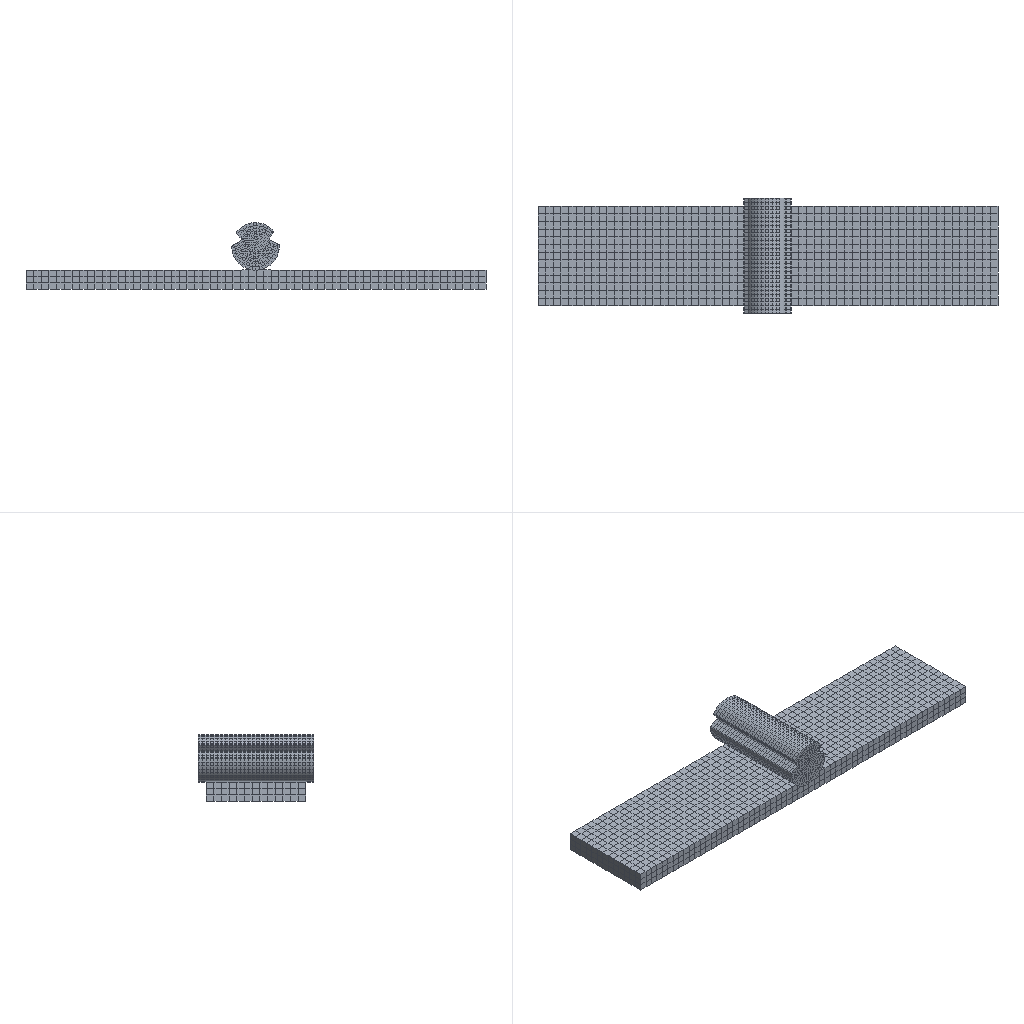Simulation study | abaqus
Set-up summary:
category,name,step,type,value,unit,region
solver,abaqus
solver,version,,,Abaqus/Standard 2020
units,not stated in the deck,,not stated
analysis,deck,,static,static
load_step,Step-1,Step-1,static
load_step,requested,,,1
mesh,nodes,,,13088
mesh,elements,,,10920
element_type,C3D8R,,solid,10920
load,load commands in deck,,count,1
bc,support commands in deck,,count,6
material,TAN,,in results
material,XIAN,,in results
check,setup vs results,,match,"per instance, exact: element labels, types and connectivity; labels of the nodes the elements use; coordinates not compared"
Abaqus input file, long lists of numbers shortened:
*Heading
** Job name: Job-2 Model name: Model-2
** Generated by: Abaqus/CAE 2020
*Preprint, echo=NO, model=NO, history=NO, contact=NO
**
** PARTS
**
*Part, name=P222
*Node
      1,         120.,         -23.,           5.
      2,         120.,         -23.,   3.333
** (3414 more lines like these left out)
*Element, type=C3D8R
   1,   57,   58,   62,   61,    1,    2,    6,    5
   2,   58,   59,   63,   62,    2,    3,    7,    6
** (2338 more lines like these left out)
*Nset, nset=Set-2, generate
    1,  3416,     1
*Elset, elset=Set-2, generate
    1,  2340,     1
** Section: tan
*Solid Section, elset=Set-2, material=tan
,
*End Part
**
*Part, name=dao
*Node
      1,   -6.104,  0.109,           0.
      2,  -5.946,  0.3737,           0.
** (9670 more lines like these left out)
*Element, type=C3D8R
   1,  164,  141,  127,  162,  476,  453,  439,  474
   2,  276,  162,  127,  277,  588,  474,  439,  589
** (8578 more lines like these left out)
*Nset, nset=Set-2, generate
    1,  9672,     1
*Elset, elset=Set-2, generate
    1,  8580,     1
** Section: xian
*Solid Section, elset=Set-2, material=xian
,
*End Part
**
**
** ASSEMBLY
**
*Assembly, name=Assembly
**
*Instance, name=P222-1, part=P222
*End Instance
**
*Instance, name=dao-1, part=dao
   59.767,           5.,    11.079
   59.767,           5.,    11.079, 60.767,           5.,    11.079, 90.
*End Instance
**
*Nset, nset=Set-1, instance=P222-1, generate
    1,  3416,     1
*Nset, nset=Set-1, instance=dao-1, generate
    1,  9672,     1
*Elset, elset=Set-1, instance=P222-1, generate
    1,  2340,     1
*Elset, elset=Set-1, instance=dao-1, generate
    1,  8580,     1
*Nset, nset=Set-2, instance=dao-1
    2,    3,    5,    6,   16,   17,   19,   20,   33,   34,   40,   41,  314,  315,  317,  318
  328,  329,  331,  332,  345,  346,  352,  353,  626,  627,  629,  630,  640,  641,  643,  644
** (22 more lines like these left out)
*Elset, elset=Set-2, instance=dao-1
   11,   28,   40,   89,   94,  175,  203,  273,  297,  314,  326,  375,  380,  461,  489,  559
  583,  600,  612,  661,  666,  747,  775,  845,  869,  886,  898,  947,  952, 1033, 1061, 1131
** (13 more lines like these left out)
*Nset, nset=Set-3, instance=P222-1, generate
    1,  3416,     1
*Nset, nset=Set-3, instance=dao-1, generate
   1,  312,    1
*Elset, elset=Set-3, instance=P222-1, generate
    1,  2340,     1
*Elset, elset=Set-3, instance=dao-1, generate
   1,  286,    1
*Nset, nset=Set-4, instance=dao-1, generate
   1,  312,    1
*Elset, elset=Set-4, instance=dao-1, generate
   1,  286,    1
*Nset, nset=Set-5, instance=P222-1
    1,    2,    3,    4,   53,   54,   55,   56,   57,   58,   59,   60,  109,  110,  111,  112
  113,  114,  115,  116,  165,  166,  167,  168,  169,  170,  171,  172,  221,  222,  223,  224
** (29 more lines like these left out)
*Elset, elset=Set-5, instance=P222-1
    1,    2,    3,   37,   38,   39,   40,   41,   42,   76,   77,   78,   79,   80,   81,  115
  116,  117,  118,  119,  120,  154,  155,  156,  157,  158,  159,  193,  194,  195,  196,  197
** (21 more lines like these left out)
*Nset, nset=Set-6, instance=P222-1, generate
    1,  3416,     1
*Nset, nset=Set-6, instance=dao-1, generate
    1,  9672,     1
*Elset, elset=Set-6, instance=P222-1, generate
    1,  2340,     1
*Elset, elset=Set-6, instance=dao-1, generate
    1,  8580,     1
*Elset, elset=_Surf-1_S2, internal, instance=dao-1, generate
 8295,  8580,     1
*Surface, type=ELEMENT, name=Surf-1
_Surf-1_S2, S2
*Elset, elset=_Surf-2_S3, internal, instance=P222-1
    1,    2,    3,   40,   41,   42,   79,   80,   81,  118,  119,  120,  157,  158,  159,  196
  197,  198,  235,  236,  237,  274,  275,  276,  313,  314,  315,  352,  353,  354,  391,  392
** (10 more lines like these left out)
*Elset, elset=_Surf-2_S3, internal, instance=dao-1
    8,   26,   63,   64,   86,   88,   89,   91,  101,  132,  147,  149,  157,  162,  179,  188
  190,  195,  197,  203,  204,  210,  217,  222,  294,  312,  349,  350,  372,  374,  375,  377
** (43 more lines like these left out)
*Elset, elset=_Surf-2_S5, internal, instance=P222-1
   37,   38,   39,   76,   77,   78,  115,  116,  117,  154,  155,  156,  193,  194,  195,  232
  233,  234,  271,  272,  273,  310,  311,  312,  349,  350,  351,  388,  389,  390,  427,  428
** (10 more lines like these left out)
*Elset, elset=_Surf-2_S5, internal, instance=dao-1
   28,   45,   54,   69,   93,  175,  191,  209,  215,  218,  220,  226,  230,  231,  233,  314
  331,  340,  355,  379,  461,  477,  495,  501,  504,  506,  512,  516,  517,  519,  600,  617
** (27 more lines like these left out)
*Elset, elset=_Surf-2_S1, internal, instance=P222-1, generate
 2302,  2340,     1
*Elset, elset=_Surf-2_S1, internal, instance=dao-1, generate
   1,  286,    1
*Elset, elset=_Surf-2_S4, internal, instance=P222-1, generate
    3,  2340,     3
*Elset, elset=_Surf-2_S4, internal, instance=dao-1
    9,   11,   33,   34,   40,   42,   94,  273,  295,  297,  319,  320,  326,  328,  380,  559
  581,  583,  605,  606,  612,  614,  666,  845,  867,  869,  891,  892,  898,  900,  952, 1131
** (13 more lines like these left out)
*Elset, elset=_Surf-2_S2, internal, instance=P222-1, generate
  1,  39,   1
*Elset, elset=_Surf-2_S2, internal, instance=dao-1, generate
 8295,  8580,     1
*Elset, elset=_Surf-2_S6, internal, instance=P222-1, generate
    1,  2338,     3
*Elset, elset=_Surf-2_S6, internal, instance=dao-1
   14,   24,   63,  300,  310,  349,  586,  596,  635,  872,  882,  921, 1158, 1168, 1207, 1444
 1454, 1493, 1730, 1740, 1779, 2016, 2026, 2065, 2302, 2312, 2351, 2588, 2598, 2637, 2874, 2884
** (4 more lines like these left out)
*Surface, type=ELEMENT, name=Surf-2
_Surf-2_S3, S3
_Surf-2_S5, S5
_Surf-2_S4, S4
_Surf-2_S2, S2
_Surf-2_S6, S6
_Surf-2_S1, S1
*Elset, elset=_Surf-3_S3, internal, instance=P222-1
    1,    2,    3,   40,   41,   42,   79,   80,   81,  118,  119,  120,  157,  158,  159,  196
  197,  198,  235,  236,  237,  274,  275,  276,  313,  314,  315,  352,  353,  354,  391,  392
** (10 more lines like these left out)
*Elset, elset=_Surf-3_S3, internal, instance=dao-1
    8,   26,   63,   64,   86,   88,   89,   91,  101,  132,  147,  149,  157,  162,  179,  188
  190,  195,  197,  203,  204,  210,  217,  222,  294,  312,  349,  350,  372,  374,  375,  377
** (43 more lines like these left out)
*Elset, elset=_Surf-3_S5, internal, instance=P222-1
   37,   38,   39,   76,   77,   78,  115,  116,  117,  154,  155,  156,  193,  194,  195,  232
  233,  234,  271,  272,  273,  310,  311,  312,  349,  350,  351,  388,  389,  390,  427,  428
** (10 more lines like these left out)
*Elset, elset=_Surf-3_S5, internal, instance=dao-1
   28,   45,   54,   69,   93,  175,  191,  209,  215,  218,  220,  226,  230,  231,  233,  314
  331,  340,  355,  379,  461,  477,  495,  501,  504,  506,  512,  516,  517,  519,  600,  617
** (27 more lines like these left out)
*Elset, elset=_Surf-3_S1, internal, instance=P222-1, generate
 2302,  2340,     1
*Elset, elset=_Surf-3_S1, internal, instance=dao-1, generate
   1,  286,    1
*Elset, elset=_Surf-3_S4, internal, instance=P222-1, generate
    3,  2340,     3
*Elset, elset=_Surf-3_S4, internal, instance=dao-1
    9,   11,   33,   34,   40,   42,   94,  273,  295,  297,  319,  320,  326,  328,  380,  559
  581,  583,  605,  606,  612,  614,  666,  845,  867,  869,  891,  892,  898,  900,  952, 1131
** (13 more lines like these left out)
*Elset, elset=_Surf-3_S2, internal, instance=P222-1, generate
  1,  39,   1
*Elset, elset=_Surf-3_S2, internal, instance=dao-1, generate
 8295,  8580,     1
*Elset, elset=_Surf-3_S6, internal, instance=P222-1, generate
    1,  2338,     3
*Elset, elset=_Surf-3_S6, internal, instance=dao-1
   14,   24,   63,  300,  310,  349,  586,  596,  635,  872,  882,  921, 1158, 1168, 1207, 1444
 1454, 1493, 1730, 1740, 1779, 2016, 2026, 2065, 2302, 2312, 2351, 2588, 2598, 2637, 2874, 2884
** (4 more lines like these left out)
*Surface, type=ELEMENT, name=Surf-3
_Surf-3_S3, S3
_Surf-3_S5, S5
_Surf-3_S4, S4
_Surf-3_S2, S2
_Surf-3_S6, S6
_Surf-3_S1, S1
*Elset, elset=_Surf-6_S4, internal, instance=P222-1, generate
    3,  2340,     3
*Surface, type=ELEMENT, name=Surf-6
_Surf-6_S4, S4
*Elset, elset=_m_Surf-4_S3, internal, instance=dao-1
   26,   86,  101,  157,  162,  179,  188,  190,  195,  197,  204,  217,  222,  312,  372,  387
  443,  448,  465,  474,  476,  481,  483,  490,  503,  508,  598,  658,  673,  729,  734,  751
** (23 more lines like these left out)
*Elset, elset=_m_Surf-4_S4, internal, instance=dao-1, generate
   33,  8327,   286
*Elset, elset=_m_Surf-4_S5, internal, instance=dao-1
   54,  191,  215,  218,  220,  226,  340,  477,  501,  504,  506,  512,  626,  763,  787,  790
  792,  798,  912, 1049, 1073, 1076, 1078, 1084, 1198, 1335, 1359, 1362, 1364, 1370, 1484, 1621
** (10 more lines like these left out)
*Surface, type=ELEMENT, name=m_Surf-4
_m_Surf-4_S3, S3
_m_Surf-4_S4, S4
_m_Surf-4_S5, S5
*Elset, elset=_s_Surf-4_S6, internal, instance=P222-1, generate
    1,  2338,     3
*Surface, type=ELEMENT, name=s_Surf-4
_s_Surf-4_S6, S6
** Constraint: Constraint-1
*Tie, name=Constraint-1, adjust=yes
s_Surf-4, m_Surf-4
*End Assembly
*Amplitude, name=Amp-1
             0.,              0.,              1.,              1.
**
** MATERIALS
**
*Material, name=tan
*Density
 1.67e-09,
*Elastic
36500., 0.425
*Expansion
 3.5e-06,
*Material, name=xian
*Density
 8.9e-09,
*Elastic
110000., 0.32
*Expansion
 1.66e-06,
*Plastic
250.,0.
**
** PHYSICAL CONSTANTS
**
*Physical Constants, absolute zero=-273., stefan boltzmann=5.67e-08
**
** BOUNDARY CONDITIONS
**
** Name: BC-1 Type: 对称/反对称/完全固定
*Boundary
Set-2, ENCASTRE
** Name: BC-3 Type: 位移/转角
*Boundary
Set-5, 2, 2
Set-5, 4, 4
Set-5, 5, 5
Set-5, 6, 6
**
** PREDEFINED FIELDS
**
** Name: Predefined Field-1   Type: Temperature
*Initial Conditions, type=TEMPERATURE
Set-1, 25.
** ----------------------------------------------------------------
**
** STEP: Step-1
**
*Step, name=Step-1, nlgeom=YES, inc=10000
*Static, stabilize=0.0002, allsdtol=0.05, continue=NO
0.001, 1., 1e-05, 1.
**
** BOUNDARY CONDITIONS
**
** Name: BC-2 Type: 电势
*Boundary
Set-4, 9, 9
**
** LOADS
**
** Name: Load-2   Type: Pressure
*Dsload, amplitude=Amp-1
Surf-6, P, 0.01
**
** PREDEFINED FIELDS
**
** Name: Predefined Field-2   Type: Temperature
*Temperature, file=D:\__________________________\_____\_____.______________________________
**
** OUTPUT REQUESTS
**
*Restart, write, frequency=0
**
** FIELD OUTPUT: F-Output-1
**
*Output, field
*Node Output
CECHG, CECUR, EPOT, NT, RF, RM, RT, TF
U, V
*Element Output, directions=YES
E, ECD, EPG, LE, MISES, PE, PEEQ, PEEQMAX, PEEQT, PEMAG, S, TEMP, VEEQ
*Contact Output
CSTRESS, ECD
**
** HISTORY OUTPUT: H-Output-1
**
*Output, history, variable=PRESELECT
*End Step
Results summary:
result,step,,completed,increments=21 time=1.0/1.0
result,analysis,,,static
result,last_loadstep,,,1
result,primary field,,,U
result,reaction total,,FX,0.003857,model units
result,reaction total,,FY,-0.000131,model units
result,reaction total,,FZ,-31.211,model units